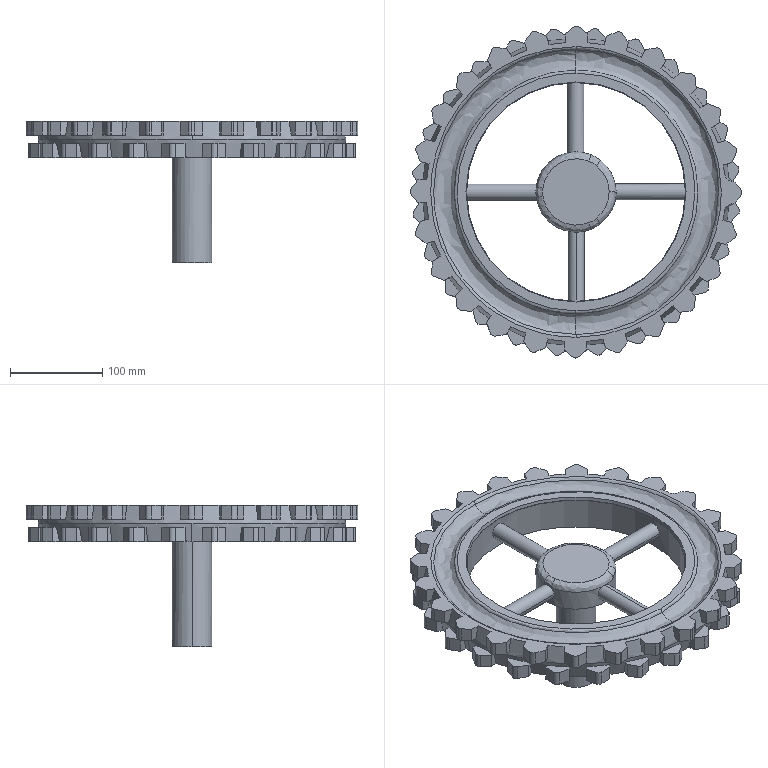Part | SolidWorks | features BaseBody 1, MoveFace 1, Scale 1 | 1 solid | 351 faces | box 360.432 x 360.432 x 153.62 mm | volume 1936645 mm3 | plane 247 | cylinder 77 | spline 21 | cone 6 | commonest cylinder face diameters 10.461 x30 10.464 x29 17.5 x8 17.22 x4 43.05 x2 87 x2